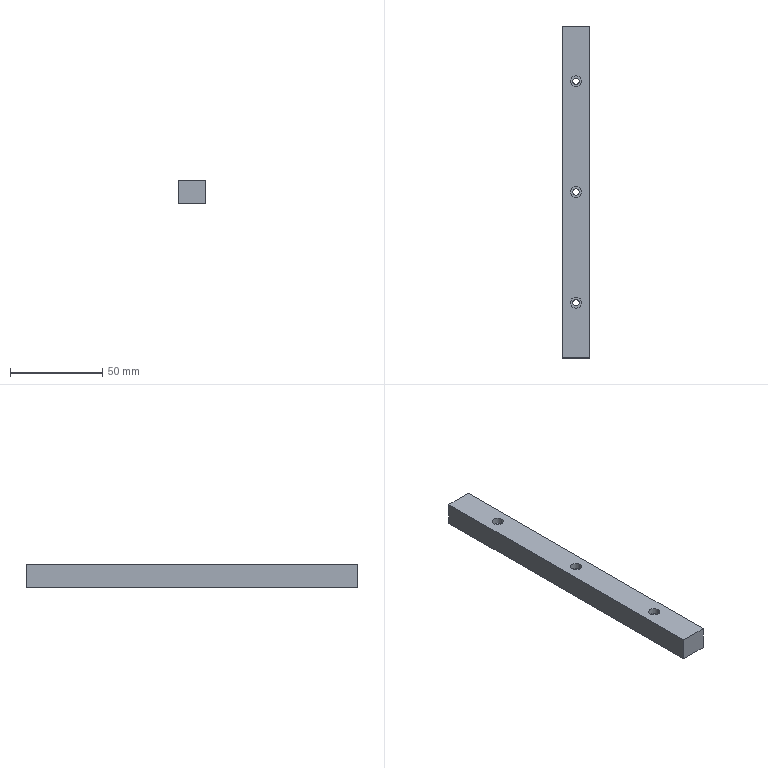Part | STEP file | Guide rail | 1 solid | 21 faces | box 15 x 180 x 12.5 mm | volume 33214 mm3 | cylinder 12 | plane 9 | commonest cylinder face diameters 3.4 x6 6 x6